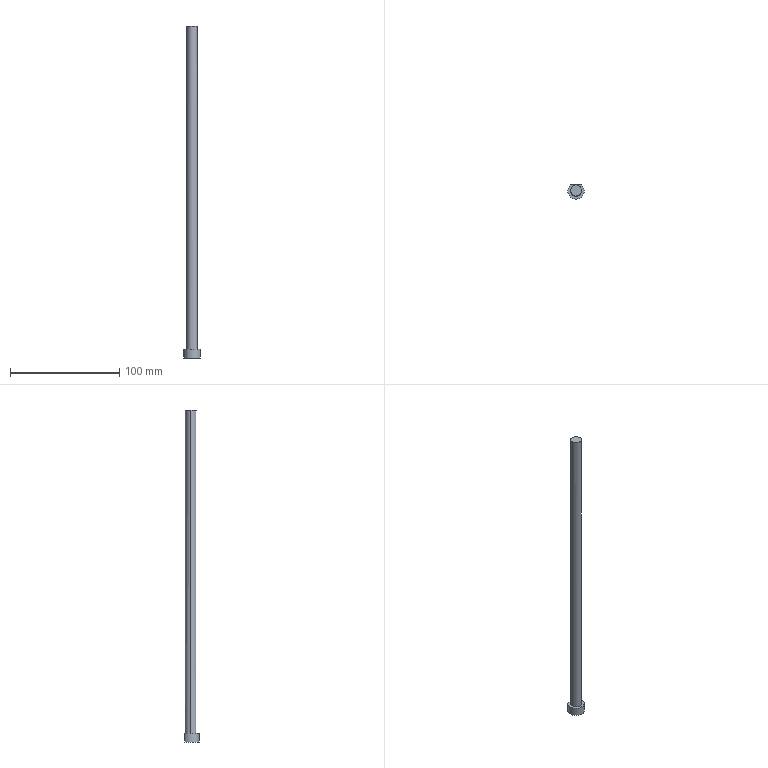Part | Creo | 1 solid | 7 faces | box 15 x 13 x 304.149 mm | volume 24556 mm3 | cylinder 4 | plane 3 | commonest cylinder face diameters 10 x2 15 x1 6839 x1
STEP:
#1=CARTESIAN_POINT('',(0.,0.,0.));
#2=DIRECTION('',(0.,0.,1.));
#3=DIRECTION('',(1.,0.,0.));
#4=AXIS2_PLACEMENT_3D('',#1,#2,#3);
#5=CARTESIAN_POINT('',(61.087,-69.161,-330.441));
#6=VERTEX_POINT('',#5);
#7=CARTESIAN_POINT('',(50.889,-69.161,-330.441));
#8=VERTEX_POINT('',#7);
#9=CARTESIAN_POINT('',(61.087,-69.161,-330.441));
#10=DIRECTION('',(-1.,0.,0.));
#11=VECTOR('',#10,10.198);
#12=LINE('',#9,#11);
#13=EDGE_CURVE('',#6,#8,#12,.T.);
#14=ORIENTED_EDGE('',*,*,#13,.F.);
#15=CARTESIAN_POINT('',(55.988,-74.661,-330.441));
#16=DIRECTION('',(0.,0.,-1.));
#17=DIRECTION('',(0.6799,0.7333,0.));
#18=AXIS2_PLACEMENT_3D('',#15,#16,#17);
#19=CIRCLE('',#18,7.5);
#20=EDGE_CURVE('',#6,#8,#19,.T.);
#21=ORIENTED_EDGE('',*,*,#20,.T.);
#22=EDGE_LOOP('',(#14,#21));
#23=FACE_OUTER_BOUND('',#22,.F.);
#24=CARTESIAN_POINT('',(50.988,-74.661,-330.441));
#25=VERTEX_POINT('',#24);
#26=CARTESIAN_POINT('',(60.988,-74.661,-330.441));
#27=VERTEX_POINT('',#26);
#28=CARTESIAN_POINT('',(55.988,-74.661,-330.441));
#29=DIRECTION('',(0.,0.,-1.));
#30=DIRECTION('',(-1.,0.,0.));
#31=AXIS2_PLACEMENT_3D('',#28,#29,#30);
#32=CIRCLE('',#31,5.);
#33=EDGE_CURVE('',#25,#27,#32,.T.);
#34=ORIENTED_EDGE('',*,*,#33,.F.);
#35=CARTESIAN_POINT('',(55.988,-74.661,-330.441));
#36=DIRECTION('',(0.,0.,-1.));
#37=DIRECTION('',(1.,0.,0.));
#38=AXIS2_PLACEMENT_3D('',#35,#36,#37);
#39=CIRCLE('',#38,5.);
#40=EDGE_CURVE('',#27,#25,#39,.T.);
#41=ORIENTED_EDGE('',*,*,#40,.F.);
#42=EDGE_LOOP('',(#34,#41));
#43=FACE_BOUND('',#42,.F.);
#44=CARTESIAN_POINT('',(55.988,-74.661,-330.441));
#45=DIRECTION('',(0.,0.,-1.));
#46=DIRECTION('',(-1.,0.,0.));
#47=AXIS2_PLACEMENT_3D('',#44,#45,#46);
#48=PLANE('',#47);
#49=ADVANCED_FACE('',(#23,#43),#48,.F.);
#50=CARTESIAN_POINT('',(60.988,-74.661,-34.416));
#51=VERTEX_POINT('',#50);
#52=CARTESIAN_POINT('',(50.988,-74.661,-34.311));
#53=VERTEX_POINT('',#52);
#54=CARTESIAN_POINT('',(60.988,-74.661,-34.416));
#55=CARTESIAN_POINT('',(60.988,-74.211,-34.42));
#56=CARTESIAN_POINT('',(60.871,-73.347,-34.427));
#57=CARTESIAN_POINT('',(60.364,-72.124,-34.432));
#58=CARTESIAN_POINT('',(59.56,-71.081,-34.432));
#59=CARTESIAN_POINT('',(58.514,-70.278,-34.427));
#60=CARTESIAN_POINT('',(57.287,-69.772,-34.418));
#61=CARTESIAN_POINT('',(55.969,-69.603,-34.406));
#62=CARTESIAN_POINT('',(54.659,-69.781,-34.39));
#63=CARTESIAN_POINT('',(53.442,-70.291,-34.374));
#64=CARTESIAN_POINT('',(52.399,-71.098,-34.356));
#65=CARTESIAN_POINT('',(51.602,-72.144,-34.339));
#66=CARTESIAN_POINT('',(51.102,-73.364,-34.324));
#67=CARTESIAN_POINT('',(50.988,-74.218,-34.315));
#68=CARTESIAN_POINT('',(50.988,-74.661,-34.311));
#69=B_SPLINE_CURVE_WITH_KNOTS('',3,(#54,#55,#56,#57,#58,#59,#60,#61,#62,#63,#64,#65,#66,#67,#68),.UNSPECIFIED.,.F.,.F.,(4,1,1,1,1,1,1,1,1,1,1,1,4),(0.,0.08333,0.1667,0.25,0.3333,0.4167,0.5,0.5833,0.6667,0.75,0.8333,0.9167,1.),.UNSPECIFIED.);
#70=EDGE_CURVE('',#51,#53,#69,.T.);
#71=ORIENTED_EDGE('',*,*,#70,.T.);
#72=CARTESIAN_POINT('',(50.988,-74.661,-330.441));
#73=DIRECTION('',(0.0000001,0.,1.));
#74=VECTOR('',#73,296.131);
#75=LINE('',#72,#74);
#76=EDGE_CURVE('',#25,#53,#75,.T.);
#77=ORIENTED_EDGE('',*,*,#76,.F.);
#78=ORIENTED_EDGE('',*,*,#33,.T.);
#79=CARTESIAN_POINT('',(60.988,-74.661,-330.441));
#80=DIRECTION('',(-0.000000051,0.,1.));
#81=VECTOR('',#80,296.025);
#82=LINE('',#79,#81);
#83=EDGE_CURVE('',#27,#51,#82,.T.);
#84=ORIENTED_EDGE('',*,*,#83,.T.);
#85=EDGE_LOOP('',(#71,#77,#78,#84));
#86=FACE_OUTER_BOUND('',#85,.F.);
#87=CARTESIAN_POINT('',(55.988,-74.661,-653.441));
#88=DIRECTION('',(0.,0.,1.));
#89=DIRECTION('',(1.,0.,0.));
#90=AXIS2_PLACEMENT_3D('',#87,#88,#89);
#91=CYLINDRICAL_SURFACE('',#90,5.);
#92=ADVANCED_FACE('',(#86),#91,.T.);
#93=CARTESIAN_POINT('',(60.987,-74.763,-34.415));
#94=VERTEX_POINT('',#93);
#95=CARTESIAN_POINT('',(50.988,-74.661,-34.311));
#96=CARTESIAN_POINT('',(50.988,-75.143,-34.306));
#97=CARTESIAN_POINT('',(51.122,-76.065,-34.299));
#98=CARTESIAN_POINT('',(51.707,-77.373,-34.292));
#99=CARTESIAN_POINT('',(52.635,-78.459,-34.291));
#100=CARTESIAN_POINT('',(53.832,-79.247,-34.296));
#101=CARTESIAN_POINT('',(55.203,-79.667,-34.306));
#102=CARTESIAN_POINT('',(56.637,-79.687,-34.321));
#103=CARTESIAN_POINT('',(58.021,-79.303,-34.339));
#104=CARTESIAN_POINT('',(59.242,-78.546,-34.36));
#105=CARTESIAN_POINT('',(60.201,-77.479,-34.381));
#106=CARTESIAN_POINT('',(60.82,-76.183,-34.4));
#107=CARTESIAN_POINT('',(60.977,-75.252,-34.411));
#108=B_SPLINE_CURVE_WITH_KNOTS('',3,(#95,#96,#97,#98,#99,#100,#101,#102,#103,#104,#105,#106,#107,#93),.UNSPECIFIED.,.F.,.F.,(4,1,1,1,1,1,1,1,1,1,1,4),(0.,0.09091,0.1818,0.2727,0.3636,0.4545,0.5455,0.6364,0.7273,0.8182,0.9091,1.),.UNSPECIFIED.);
#109=EDGE_CURVE('',#53,#94,#108,.T.);
#110=ORIENTED_EDGE('',*,*,#109,.F.);
#111=ORIENTED_EDGE('',*,*,#70,.F.);
#112=CARTESIAN_POINT('',(60.987,-74.763,-34.415));
#113=CARTESIAN_POINT('',(60.987,-74.752,-34.415));
#114=CARTESIAN_POINT('',(60.988,-74.729,-34.416));
#115=CARTESIAN_POINT('',(60.988,-74.695,-34.416));
#116=CARTESIAN_POINT('',(60.988,-74.672,-34.416));
#117=CARTESIAN_POINT('',(60.988,-74.661,-34.416));
#118=B_SPLINE_CURVE_WITH_KNOTS('',3,(#112,#113,#114,#115,#116,#117),.UNSPECIFIED.,.F.,.F.,(4,1,1,4),(0.,0.3333,0.6667,1.),.UNSPECIFIED.);
#119=EDGE_CURVE('',#94,#51,#118,.T.);
#120=ORIENTED_EDGE('',*,*,#119,.F.);
#121=EDGE_LOOP('',(#110,#111,#120));
#122=FACE_OUTER_BOUND('',#121,.F.);
#123=CARTESIAN_POINT('',(19.928,-102.127,-3453.443));
#124=DIRECTION('',(0.009422,0.9999,-0.009215));
#125=DIRECTION('',(0.01202,0.009102,0.9999));
#126=AXIS2_PLACEMENT_3D('',#123,#124,#125);
#127=CYLINDRICAL_SURFACE('',#126,3419.382);
#128=ADVANCED_FACE('',(#122),#127,.T.);
#129=ORIENTED_EDGE('',*,*,#109,.T.);
#130=ORIENTED_EDGE('',*,*,#119,.T.);
#131=ORIENTED_EDGE('',*,*,#83,.F.);
#132=ORIENTED_EDGE('',*,*,#40,.T.);
#133=ORIENTED_EDGE('',*,*,#76,.T.);
#134=EDGE_LOOP('',(#129,#130,#131,#132,#133));
#135=FACE_OUTER_BOUND('',#134,.F.);
#136=CARTESIAN_POINT('',(55.988,-74.661,-653.441));
#137=DIRECTION('',(0.,0.,1.));
#138=DIRECTION('',(1.,0.,0.));
#139=AXIS2_PLACEMENT_3D('',#136,#137,#138);
#140=CYLINDRICAL_SURFACE('',#139,5.);
#141=ADVANCED_FACE('',(#135),#140,.T.);
#142=CARTESIAN_POINT('',(50.889,-69.161,-338.441));
#143=VERTEX_POINT('',#142);
#144=CARTESIAN_POINT('',(50.889,-69.161,-330.441));
#145=DIRECTION('',(0.,0.,-1.));
#146=VECTOR('',#145,8.);
#147=LINE('',#144,#146);
#148=EDGE_CURVE('',#8,#143,#147,.T.);
#149=ORIENTED_EDGE('',*,*,#148,.T.);
#150=CARTESIAN_POINT('',(61.087,-69.161,-338.441));
#151=VERTEX_POINT('',#150);
#152=CARTESIAN_POINT('',(61.087,-69.161,-338.441));
#153=DIRECTION('',(-1.,0.,0.));
#154=VECTOR('',#153,10.198);
#155=LINE('',#152,#154);
#156=EDGE_CURVE('',#151,#143,#155,.T.);
#157=ORIENTED_EDGE('',*,*,#156,.F.);
#158=CARTESIAN_POINT('',(61.087,-69.161,-338.441));
#159=DIRECTION('',(0.,0.,1.));
#160=VECTOR('',#159,8.);
#161=LINE('',#158,#160);
#162=EDGE_CURVE('',#151,#6,#161,.T.);
#163=ORIENTED_EDGE('',*,*,#162,.T.);
#164=ORIENTED_EDGE('',*,*,#13,.T.);
#165=EDGE_LOOP('',(#149,#157,#163,#164));
#166=FACE_OUTER_BOUND('',#165,.F.);
#167=CARTESIAN_POINT('',(55.988,-69.161,-338.441));
#168=DIRECTION('',(0.,1.,0.));
#169=DIRECTION('',(0.,0.,1.));
#170=AXIS2_PLACEMENT_3D('',#167,#168,#169);
#171=PLANE('',#170);
#172=ADVANCED_FACE('',(#166),#171,.T.);
#173=CARTESIAN_POINT('',(55.988,-74.661,-338.441));
#174=DIRECTION('',(0.,0.,1.));
#175=DIRECTION('',(-0.6799,0.7333,0.));
#176=AXIS2_PLACEMENT_3D('',#173,#174,#175);
#177=CIRCLE('',#176,7.5);
#178=EDGE_CURVE('',#143,#151,#177,.T.);
#179=ORIENTED_EDGE('',*,*,#178,.F.);
#180=ORIENTED_EDGE('',*,*,#148,.F.);
#181=ORIENTED_EDGE('',*,*,#20,.F.);
#182=ORIENTED_EDGE('',*,*,#162,.F.);
#183=EDGE_LOOP('',(#179,#180,#181,#182));
#184=FACE_OUTER_BOUND('',#183,.F.);
#185=CARTESIAN_POINT('',(55.988,-74.661,-330.441));
#186=DIRECTION('',(0.,0.,-1.));
#187=DIRECTION('',(-1.,0.,0.));
#188=AXIS2_PLACEMENT_3D('',#185,#186,#187);
#189=CYLINDRICAL_SURFACE('',#188,7.5);
#190=ADVANCED_FACE('',(#184),#189,.T.);
#191=ORIENTED_EDGE('',*,*,#178,.T.);
#192=ORIENTED_EDGE('',*,*,#156,.T.);
#193=EDGE_LOOP('',(#191,#192));
#194=FACE_OUTER_BOUND('',#193,.F.);
#195=CARTESIAN_POINT('',(71.601,-78.127,-338.441));
#196=DIRECTION('',(0.,0.,-1.));
#197=DIRECTION('',(-1.,0.,0.));
#198=AXIS2_PLACEMENT_3D('',#195,#196,#197);
#199=PLANE('',#198);
#200=ADVANCED_FACE('',(#194),#199,.T.);
#201=CLOSED_SHELL('',(#49,#92,#128,#141,#172,#190,#200));
#202=MANIFOLD_SOLID_BREP('',#201);
#203=(LENGTH_UNIT()NAMED_UNIT(*)SI_UNIT(.MILLI.,.METRE.));
#204=UNCERTAINTY_MEASURE_WITH_UNIT(LENGTH_MEASURE(0.03048),#203,'','');
#205=(NAMED_UNIT(*)PLANE_ANGLE_UNIT()SI_UNIT($,.RADIAN.));
#206=PLANE_ANGLE_MEASURE_WITH_UNIT(PLANE_ANGLE_MEASURE(0.01745),#205);
#207=(CONVERSION_BASED_UNIT('DEGREE',#206)NAMED_UNIT(*)PLANE_ANGLE_UNIT());
#208=(NAMED_UNIT(*)SI_UNIT($,.STERADIAN.)SOLID_ANGLE_UNIT());
#209=(GEOMETRIC_REPRESENTATION_CONTEXT(3)GLOBAL_UNCERTAINTY_ASSIGNED_CONTEXT((#204))GLOBAL_UNIT_ASSIGNED_CONTEXT((#203,#207,#208))REPRESENTATION_CONTEXT('',''));
#210=ADVANCED_BREP_SHAPE_REPRESENTATION('',(#4,#202),#209);